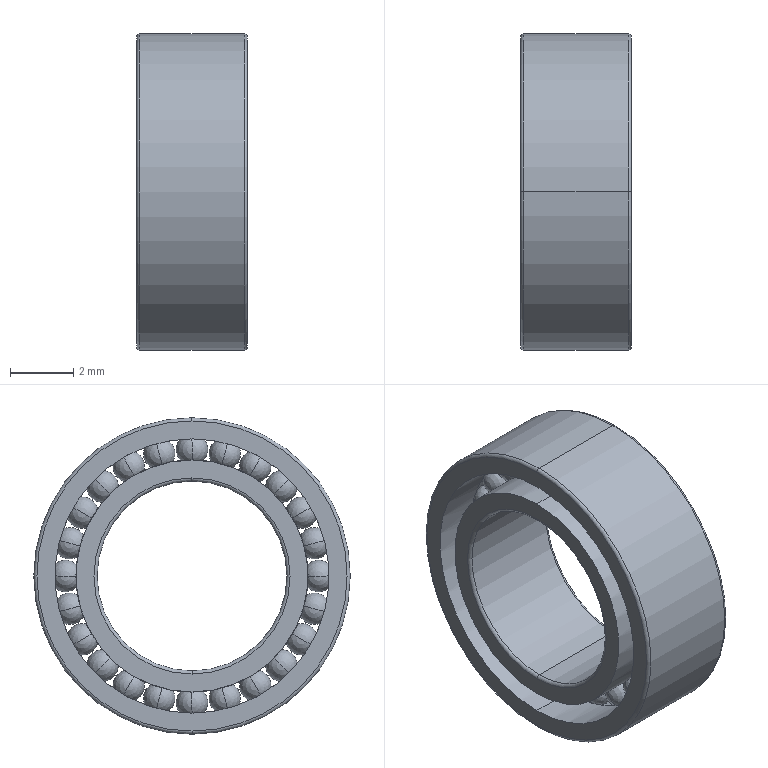Part | SolidWorks | features BaseBody 1 | 1 solid | 192 faces | box 3.5 x 10 x 10 mm | volume 125.675 mm3 | sphere 96 | torus 80 | cylinder 12 | plane 4 | commonest cylinder face diameters 7.333 x4 8.667 x4 6 x2 10 x2